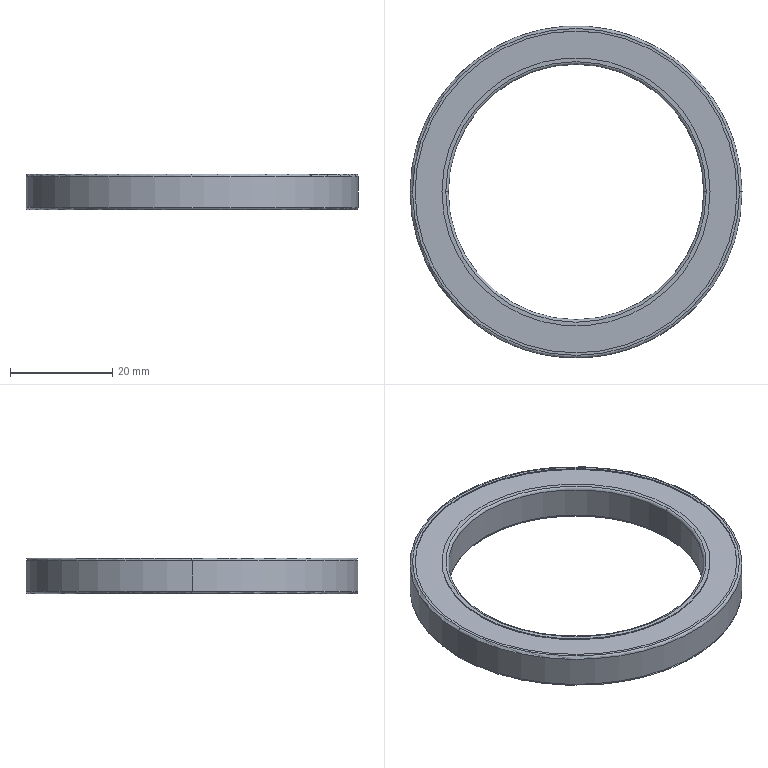Part | SolidWorks | features Extrusion 1, Fillet 1, ICE 1, MirrorPattern 1 | 1 solid | 26 faces | box 65 x 65 x 7 mm | volume 9064 mm3 | cylinder 12 | torus 8 | plane 6 | commonest cylinder face diameters 52.5 x4 63 x4 50 x2 65 x2
STEP:
#1=CARTESIAN_POINT('',(-25.5,0.,3.5));
#2=VERTEX_POINT('',#1);
#3=CARTESIAN_POINT('',(25.5,0.,3.5));
#4=VERTEX_POINT('',#3);
#5=CARTESIAN_POINT('',(0.,0.,3.5));
#6=DIRECTION('',(0.,0.,-1.));
#7=DIRECTION('',(1.,0.,0.));
#8=AXIS2_PLACEMENT_3D('',#5,#6,#7);
#9=CIRCLE('',#8,25.5);
#10=EDGE_CURVE('',#2,#4,#9,.T.);
#11=ORIENTED_EDGE('',*,*,#10,.F.);
#12=CARTESIAN_POINT('',(-25.,0.,3.));
#13=VERTEX_POINT('',#12);
#14=CARTESIAN_POINT('',(-25.5,0.,3.));
#15=DIRECTION('',(0.,1.,0.));
#16=DIRECTION('',(-1.,0.,0.));
#17=AXIS2_PLACEMENT_3D('',#14,#15,#16);
#18=CIRCLE('',#17,0.5);
#19=EDGE_CURVE('',#2,#13,#18,.T.);
#20=ORIENTED_EDGE('',*,*,#19,.T.);
#21=CARTESIAN_POINT('',(25.,0.,3.));
#22=VERTEX_POINT('',#21);
#23=CARTESIAN_POINT('',(0.,0.,3.));
#24=DIRECTION('',(0.,0.,1.));
#25=DIRECTION('',(1.,0.,0.));
#26=AXIS2_PLACEMENT_3D('',#23,#24,#25);
#27=CIRCLE('',#26,25.);
#28=EDGE_CURVE('',#22,#13,#27,.T.);
#29=ORIENTED_EDGE('',*,*,#28,.F.);
#30=CARTESIAN_POINT('',(25.5,0.,3.));
#31=DIRECTION('',(0.,-1.,0.));
#32=DIRECTION('',(0.,0.,-1.));
#33=AXIS2_PLACEMENT_3D('',#30,#31,#32);
#34=CIRCLE('',#33,0.5);
#35=EDGE_CURVE('',#4,#22,#34,.T.);
#36=ORIENTED_EDGE('',*,*,#35,.F.);
#37=EDGE_LOOP('',(#11,#20,#29,#36));
#38=FACE_OUTER_BOUND('',#37,.T.);
#39=CARTESIAN_POINT('',(0.,0.,3.));
#40=DIRECTION('',(0.,0.,1.));
#41=DIRECTION('',(1.,0.,0.));
#42=AXIS2_PLACEMENT_3D('',#39,#40,#41);
#43=TOROIDAL_SURFACE('',#42,25.5,0.5);
#44=ADVANCED_FACE('',(#38),#43,.T.);
#45=CARTESIAN_POINT('',(-25.,0.,-3.));
#46=VERTEX_POINT('',#45);
#47=CARTESIAN_POINT('',(25.,0.,-3.));
#48=VERTEX_POINT('',#47);
#49=CARTESIAN_POINT('',(0.,0.,-3.));
#50=DIRECTION('',(0.,0.,-1.));
#51=DIRECTION('',(1.,0.,0.));
#52=AXIS2_PLACEMENT_3D('',#49,#50,#51);
#53=CIRCLE('',#52,25.);
#54=EDGE_CURVE('',#46,#48,#53,.T.);
#55=ORIENTED_EDGE('',*,*,#54,.F.);
#56=CARTESIAN_POINT('',(-25.5,0.,-3.5));
#57=VERTEX_POINT('',#56);
#58=CARTESIAN_POINT('',(-25.5,0.,-3.));
#59=DIRECTION('',(0.,1.,0.));
#60=DIRECTION('',(-1.,0.,0.));
#61=AXIS2_PLACEMENT_3D('',#58,#59,#60);
#62=CIRCLE('',#61,0.5);
#63=EDGE_CURVE('',#46,#57,#62,.T.);
#64=ORIENTED_EDGE('',*,*,#63,.T.);
#65=CARTESIAN_POINT('',(25.5,0.,-3.5));
#66=VERTEX_POINT('',#65);
#67=CARTESIAN_POINT('',(0.,0.,-3.5));
#68=DIRECTION('',(0.,0.,1.));
#69=DIRECTION('',(1.,0.,0.));
#70=AXIS2_PLACEMENT_3D('',#67,#68,#69);
#71=CIRCLE('',#70,25.5);
#72=EDGE_CURVE('',#66,#57,#71,.T.);
#73=ORIENTED_EDGE('',*,*,#72,.F.);
#74=CARTESIAN_POINT('',(25.5,0.,-3.));
#75=DIRECTION('',(0.,-1.,0.));
#76=DIRECTION('',(0.,0.,-1.));
#77=AXIS2_PLACEMENT_3D('',#74,#75,#76);
#78=CIRCLE('',#77,0.5);
#79=EDGE_CURVE('',#48,#66,#78,.T.);
#80=ORIENTED_EDGE('',*,*,#79,.F.);
#81=EDGE_LOOP('',(#55,#64,#73,#80));
#82=FACE_OUTER_BOUND('',#81,.T.);
#83=CARTESIAN_POINT('',(0.,0.,-3.));
#84=DIRECTION('',(0.,0.,1.));
#85=DIRECTION('',(1.,0.,0.));
#86=AXIS2_PLACEMENT_3D('',#83,#84,#85);
#87=TOROIDAL_SURFACE('',#86,25.5,0.5);
#88=ADVANCED_FACE('',(#82),#87,.T.);
#89=CARTESIAN_POINT('',(-32.5,0.,3.));
#90=VERTEX_POINT('',#89);
#91=CARTESIAN_POINT('',(32.5,0.,3.));
#92=VERTEX_POINT('',#91);
#93=CARTESIAN_POINT('',(0.,0.,3.));
#94=DIRECTION('',(0.,0.,-1.));
#95=DIRECTION('',(1.,0.,0.));
#96=AXIS2_PLACEMENT_3D('',#93,#94,#95);
#97=CIRCLE('',#96,32.5);
#98=EDGE_CURVE('',#90,#92,#97,.T.);
#99=ORIENTED_EDGE('',*,*,#98,.F.);
#100=CARTESIAN_POINT('',(-32.,0.,3.5));
#101=VERTEX_POINT('',#100);
#102=CARTESIAN_POINT('',(-32.,0.,3.));
#103=DIRECTION('',(0.,1.,0.));
#104=DIRECTION('',(-1.,0.,0.));
#105=AXIS2_PLACEMENT_3D('',#102,#103,#104);
#106=CIRCLE('',#105,0.5);
#107=EDGE_CURVE('',#90,#101,#106,.T.);
#108=ORIENTED_EDGE('',*,*,#107,.T.);
#109=CARTESIAN_POINT('',(32.,0.,3.5));
#110=VERTEX_POINT('',#109);
#111=CARTESIAN_POINT('',(0.,0.,3.5));
#112=DIRECTION('',(0.,0.,1.));
#113=DIRECTION('',(1.,0.,0.));
#114=AXIS2_PLACEMENT_3D('',#111,#112,#113);
#115=CIRCLE('',#114,32.);
#116=EDGE_CURVE('',#110,#101,#115,.T.);
#117=ORIENTED_EDGE('',*,*,#116,.F.);
#118=CARTESIAN_POINT('',(32.,0.,3.));
#119=DIRECTION('',(0.,-1.,0.));
#120=DIRECTION('',(0.,0.,-1.));
#121=AXIS2_PLACEMENT_3D('',#118,#119,#120);
#122=CIRCLE('',#121,0.5);
#123=EDGE_CURVE('',#92,#110,#122,.T.);
#124=ORIENTED_EDGE('',*,*,#123,.F.);
#125=EDGE_LOOP('',(#99,#108,#117,#124));
#126=FACE_OUTER_BOUND('',#125,.T.);
#127=CARTESIAN_POINT('',(0.,0.,3.));
#128=DIRECTION('',(0.,0.,1.));
#129=DIRECTION('',(1.,0.,0.));
#130=AXIS2_PLACEMENT_3D('',#127,#128,#129);
#131=TOROIDAL_SURFACE('',#130,32.,0.5);
#132=ADVANCED_FACE('',(#126),#131,.T.);
#133=CARTESIAN_POINT('',(-32.,0.,-3.5));
#134=VERTEX_POINT('',#133);
#135=CARTESIAN_POINT('',(32.,0.,-3.5));
#136=VERTEX_POINT('',#135);
#137=CARTESIAN_POINT('',(0.,0.,-3.5));
#138=DIRECTION('',(0.,0.,-1.));
#139=DIRECTION('',(1.,0.,0.));
#140=AXIS2_PLACEMENT_3D('',#137,#138,#139);
#141=CIRCLE('',#140,32.);
#142=EDGE_CURVE('',#134,#136,#141,.T.);
#143=ORIENTED_EDGE('',*,*,#142,.F.);
#144=CARTESIAN_POINT('',(-32.5,0.,-3.));
#145=VERTEX_POINT('',#144);
#146=CARTESIAN_POINT('',(-32.,0.,-3.));
#147=DIRECTION('',(0.,1.,0.));
#148=DIRECTION('',(-1.,0.,0.));
#149=AXIS2_PLACEMENT_3D('',#146,#147,#148);
#150=CIRCLE('',#149,0.5);
#151=EDGE_CURVE('',#134,#145,#150,.T.);
#152=ORIENTED_EDGE('',*,*,#151,.T.);
#153=CARTESIAN_POINT('',(32.5,0.,-3.));
#154=VERTEX_POINT('',#153);
#155=CARTESIAN_POINT('',(0.,0.,-3.));
#156=DIRECTION('',(0.,0.,1.));
#157=DIRECTION('',(1.,0.,0.));
#158=AXIS2_PLACEMENT_3D('',#155,#156,#157);
#159=CIRCLE('',#158,32.5);
#160=EDGE_CURVE('',#154,#145,#159,.T.);
#161=ORIENTED_EDGE('',*,*,#160,.F.);
#162=CARTESIAN_POINT('',(32.,0.,-3.));
#163=DIRECTION('',(0.,-1.,0.));
#164=DIRECTION('',(0.,0.,-1.));
#165=AXIS2_PLACEMENT_3D('',#162,#163,#164);
#166=CIRCLE('',#165,0.5);
#167=EDGE_CURVE('',#136,#154,#166,.T.);
#168=ORIENTED_EDGE('',*,*,#167,.F.);
#169=EDGE_LOOP('',(#143,#152,#161,#168));
#170=FACE_OUTER_BOUND('',#169,.T.);
#171=CARTESIAN_POINT('',(0.,0.,-3.));
#172=DIRECTION('',(0.,0.,1.));
#173=DIRECTION('',(1.,0.,0.));
#174=AXIS2_PLACEMENT_3D('',#171,#172,#173);
#175=TOROIDAL_SURFACE('',#174,32.,0.5);
#176=ADVANCED_FACE('',(#170),#175,.T.);
#177=CARTESIAN_POINT('',(26.25,0.,-3.3));
#178=VERTEX_POINT('',#177);
#179=CARTESIAN_POINT('',(-26.25,0.,-3.3));
#180=VERTEX_POINT('',#179);
#181=CARTESIAN_POINT('',(0.,0.,-3.3));
#182=DIRECTION('',(0.,0.,1.));
#183=DIRECTION('',(1.,0.,0.));
#184=AXIS2_PLACEMENT_3D('',#181,#182,#183);
#185=CIRCLE('',#184,26.25);
#186=EDGE_CURVE('',#178,#180,#185,.T.);
#187=ORIENTED_EDGE('',*,*,#186,.F.);
#188=CARTESIAN_POINT('',(26.25,0.,-3.5));
#189=VERTEX_POINT('',#188);
#190=CARTESIAN_POINT('',(26.25,0.,-3.3));
#191=DIRECTION('',(0.,0.,-1.));
#192=VECTOR('',#191,1000.);
#193=LINE('',#190,#192);
#194=EDGE_CURVE('',#178,#189,#193,.T.);
#195=ORIENTED_EDGE('',*,*,#194,.T.);
#196=CARTESIAN_POINT('',(-26.25,0.,-3.5));
#197=VERTEX_POINT('',#196);
#198=CARTESIAN_POINT('',(0.,0.,-3.5));
#199=DIRECTION('',(0.,0.,1.));
#200=DIRECTION('',(1.,0.,0.));
#201=AXIS2_PLACEMENT_3D('',#198,#199,#200);
#202=CIRCLE('',#201,26.25);
#203=EDGE_CURVE('',#189,#197,#202,.T.);
#204=ORIENTED_EDGE('',*,*,#203,.T.);
#205=CARTESIAN_POINT('',(-26.25,0.,-3.3));
#206=DIRECTION('',(0.,0.,-1.));
#207=VECTOR('',#206,1000.);
#208=LINE('',#205,#207);
#209=EDGE_CURVE('',#180,#197,#208,.T.);
#210=ORIENTED_EDGE('',*,*,#209,.F.);
#211=EDGE_LOOP('',(#187,#195,#204,#210));
#212=FACE_OUTER_BOUND('',#211,.T.);
#213=CARTESIAN_POINT('',(0.,0.,-3.3));
#214=DIRECTION('',(0.,0.,-1.));
#215=DIRECTION('',(-1.,0.,0.));
#216=AXIS2_PLACEMENT_3D('',#213,#214,#215);
#217=CYLINDRICAL_SURFACE('',#216,26.25);
#218=ADVANCED_FACE('',(#212),#217,.T.);
#219=CARTESIAN_POINT('',(-31.5,0.,-3.3));
#220=VERTEX_POINT('',#219);
#221=CARTESIAN_POINT('',(31.5,0.,-3.3));
#222=VERTEX_POINT('',#221);
#223=CARTESIAN_POINT('',(0.,0.,-3.3));
#224=DIRECTION('',(0.,0.,1.));
#225=DIRECTION('',(1.,0.,0.));
#226=AXIS2_PLACEMENT_3D('',#223,#224,#225);
#227=CIRCLE('',#226,31.5);
#228=EDGE_CURVE('',#220,#222,#227,.T.);
#229=ORIENTED_EDGE('',*,*,#228,.T.);
#230=CARTESIAN_POINT('',(31.5,0.,-3.5));
#231=VERTEX_POINT('',#230);
#232=CARTESIAN_POINT('',(31.5,0.,-3.3));
#233=DIRECTION('',(0.,0.,-1.));
#234=VECTOR('',#233,1000.);
#235=LINE('',#232,#234);
#236=EDGE_CURVE('',#222,#231,#235,.T.);
#237=ORIENTED_EDGE('',*,*,#236,.T.);
#238=CARTESIAN_POINT('',(-31.5,0.,-3.5));
#239=VERTEX_POINT('',#238);
#240=CARTESIAN_POINT('',(0.,0.,-3.5));
#241=DIRECTION('',(0.,0.,1.));
#242=DIRECTION('',(1.,0.,0.));
#243=AXIS2_PLACEMENT_3D('',#240,#241,#242);
#244=CIRCLE('',#243,31.5);
#245=EDGE_CURVE('',#239,#231,#244,.T.);
#246=ORIENTED_EDGE('',*,*,#245,.F.);
#247=CARTESIAN_POINT('',(-31.5,0.,-3.3));
#248=DIRECTION('',(0.,0.,-1.));
#249=VECTOR('',#248,1000.);
#250=LINE('',#247,#249);
#251=EDGE_CURVE('',#220,#239,#250,.T.);
#252=ORIENTED_EDGE('',*,*,#251,.F.);
#253=EDGE_LOOP('',(#229,#237,#246,#252));
#254=FACE_OUTER_BOUND('',#253,.T.);
#255=CARTESIAN_POINT('',(0.,0.,-3.3));
#256=DIRECTION('',(0.,0.,-1.));
#257=DIRECTION('',(-1.,0.,0.));
#258=AXIS2_PLACEMENT_3D('',#255,#256,#257);
#259=CYLINDRICAL_SURFACE('',#258,31.5);
#260=ADVANCED_FACE('',(#254),#259,.F.);
#261=CARTESIAN_POINT('',(26.25,0.,3.3));
#262=VERTEX_POINT('',#261);
#263=CARTESIAN_POINT('',(-26.25,0.,3.3));
#264=VERTEX_POINT('',#263);
#265=CARTESIAN_POINT('',(0.,0.,3.3));
#266=DIRECTION('',(0.,0.,1.));
#267=DIRECTION('',(1.,0.,0.));
#268=AXIS2_PLACEMENT_3D('',#265,#266,#267);
#269=CIRCLE('',#268,26.25);
#270=EDGE_CURVE('',#262,#264,#269,.T.);
#271=ORIENTED_EDGE('',*,*,#270,.T.);
#272=CARTESIAN_POINT('',(-26.25,0.,3.5));
#273=VERTEX_POINT('',#272);
#274=CARTESIAN_POINT('',(-26.25,0.,3.3));
#275=DIRECTION('',(0.,0.,1.));
#276=VECTOR('',#275,1000.);
#277=LINE('',#274,#276);
#278=EDGE_CURVE('',#264,#273,#277,.T.);
#279=ORIENTED_EDGE('',*,*,#278,.T.);
#280=CARTESIAN_POINT('',(26.25,0.,3.5));
#281=VERTEX_POINT('',#280);
#282=CARTESIAN_POINT('',(0.,0.,3.5));
#283=DIRECTION('',(0.,0.,1.));
#284=DIRECTION('',(1.,0.,0.));
#285=AXIS2_PLACEMENT_3D('',#282,#283,#284);
#286=CIRCLE('',#285,26.25);
#287=EDGE_CURVE('',#281,#273,#286,.T.);
#288=ORIENTED_EDGE('',*,*,#287,.F.);
#289=CARTESIAN_POINT('',(26.25,0.,3.3));
#290=DIRECTION('',(0.,0.,1.));
#291=VECTOR('',#290,1000.);
#292=LINE('',#289,#291);
#293=EDGE_CURVE('',#262,#281,#292,.T.);
#294=ORIENTED_EDGE('',*,*,#293,.F.);
#295=EDGE_LOOP('',(#271,#279,#288,#294));
#296=FACE_OUTER_BOUND('',#295,.T.);
#297=CARTESIAN_POINT('',(0.,0.,3.3));
#298=DIRECTION('',(0.,0.,1.));
#299=DIRECTION('',(1.,0.,0.));
#300=AXIS2_PLACEMENT_3D('',#297,#298,#299);
#301=CYLINDRICAL_SURFACE('',#300,26.25);
#302=ADVANCED_FACE('',(#296),#301,.T.);
#303=CARTESIAN_POINT('',(-31.5,0.,3.3));
#304=VERTEX_POINT('',#303);
#305=CARTESIAN_POINT('',(31.5,0.,3.3));
#306=VERTEX_POINT('',#305);
#307=CARTESIAN_POINT('',(0.,0.,3.3));
#308=DIRECTION('',(0.,0.,1.));
#309=DIRECTION('',(1.,0.,0.));
#310=AXIS2_PLACEMENT_3D('',#307,#308,#309);
#311=CIRCLE('',#310,31.5);
#312=EDGE_CURVE('',#304,#306,#311,.T.);
#313=ORIENTED_EDGE('',*,*,#312,.F.);
#314=CARTESIAN_POINT('',(-31.5,0.,3.5));
#315=VERTEX_POINT('',#314);
#316=CARTESIAN_POINT('',(-31.5,0.,3.3));
#317=DIRECTION('',(0.,0.,1.));
#318=VECTOR('',#317,1000.);
#319=LINE('',#316,#318);
#320=EDGE_CURVE('',#304,#315,#319,.T.);
#321=ORIENTED_EDGE('',*,*,#320,.T.);
#322=CARTESIAN_POINT('',(31.5,0.,3.5));
#323=VERTEX_POINT('',#322);
#324=CARTESIAN_POINT('',(0.,0.,3.5));
#325=DIRECTION('',(0.,0.,1.));
#326=DIRECTION('',(1.,0.,0.));
#327=AXIS2_PLACEMENT_3D('',#324,#325,#326);
#328=CIRCLE('',#327,31.5);
#329=EDGE_CURVE('',#315,#323,#328,.T.);
#330=ORIENTED_EDGE('',*,*,#329,.T.);
#331=CARTESIAN_POINT('',(31.5,0.,3.3));
#332=DIRECTION('',(0.,0.,1.));
#333=VECTOR('',#332,1000.);
#334=LINE('',#331,#333);
#335=EDGE_CURVE('',#306,#323,#334,.T.);
#336=ORIENTED_EDGE('',*,*,#335,.F.);
#337=EDGE_LOOP('',(#313,#321,#330,#336));
#338=FACE_OUTER_BOUND('',#337,.T.);
#339=CARTESIAN_POINT('',(0.,0.,3.3));
#340=DIRECTION('',(0.,0.,1.));
#341=DIRECTION('',(1.,0.,0.));
#342=AXIS2_PLACEMENT_3D('',#339,#340,#341);
#343=CYLINDRICAL_SURFACE('',#342,31.5);
#344=ADVANCED_FACE('',(#338),#343,.F.);
#345=CARTESIAN_POINT('',(0.,0.,3.));
#346=DIRECTION('',(0.,0.,1.));
#347=DIRECTION('',(1.,0.,0.));
#348=AXIS2_PLACEMENT_3D('',#345,#346,#347);
#349=CIRCLE('',#348,25.);
#350=EDGE_CURVE('',#13,#22,#349,.T.);
#351=ORIENTED_EDGE('',*,*,#350,.T.);
#352=CARTESIAN_POINT('',(25.,0.,3.5));
#353=DIRECTION('',(0.,0.,-1.));
#354=VECTOR('',#353,1000.);
#355=LINE('',#352,#354);
#356=EDGE_CURVE('',#22,#48,#355,.T.);
#357=ORIENTED_EDGE('',*,*,#356,.T.);
#358=CARTESIAN_POINT('',(0.,0.,-3.));
#359=DIRECTION('',(0.,0.,-1.));
#360=DIRECTION('',(1.,0.,0.));
#361=AXIS2_PLACEMENT_3D('',#358,#359,#360);
#362=CIRCLE('',#361,25.);
#363=EDGE_CURVE('',#48,#46,#362,.T.);
#364=ORIENTED_EDGE('',*,*,#363,.T.);
#365=CARTESIAN_POINT('',(-25.,0.,3.5));
#366=DIRECTION('',(0.,0.,-1.));
#367=VECTOR('',#366,1000.);
#368=LINE('',#365,#367);
#369=EDGE_CURVE('',#13,#46,#368,.T.);
#370=ORIENTED_EDGE('',*,*,#369,.F.);
#371=EDGE_LOOP('',(#351,#357,#364,#370));
#372=FACE_OUTER_BOUND('',#371,.T.);
#373=CARTESIAN_POINT('',(0.,0.,3.5));
#374=DIRECTION('',(0.,0.,-1.));
#375=DIRECTION('',(-1.,0.,0.));
#376=AXIS2_PLACEMENT_3D('',#373,#374,#375);
#377=CYLINDRICAL_SURFACE('',#376,25.);
#378=ADVANCED_FACE('',(#372),#377,.F.);
#379=ORIENTED_EDGE('',*,*,#98,.T.);
#380=CARTESIAN_POINT('',(32.5,0.,3.5));
#381=DIRECTION('',(0.,0.,-1.));
#382=VECTOR('',#381,1000.);
#383=LINE('',#380,#382);
#384=EDGE_CURVE('',#92,#154,#383,.T.);
#385=ORIENTED_EDGE('',*,*,#384,.T.);
#386=ORIENTED_EDGE('',*,*,#160,.T.);
#387=CARTESIAN_POINT('',(-32.5,0.,3.5));
#388=DIRECTION('',(0.,0.,-1.));
#389=VECTOR('',#388,1000.);
#390=LINE('',#387,#389);
#391=EDGE_CURVE('',#90,#145,#390,.T.);
#392=ORIENTED_EDGE('',*,*,#391,.F.);
#393=EDGE_LOOP('',(#379,#385,#386,#392));
#394=FACE_OUTER_BOUND('',#393,.T.);
#395=CARTESIAN_POINT('',(0.,0.,3.5));
#396=DIRECTION('',(0.,0.,-1.));
#397=DIRECTION('',(-1.,0.,0.));
#398=AXIS2_PLACEMENT_3D('',#395,#396,#397);
#399=CYLINDRICAL_SURFACE('',#398,32.5);
#400=ADVANCED_FACE('',(#394),#399,.T.);
#401=CARTESIAN_POINT('',(0.,0.,-3.5));
#402=DIRECTION('',(0.,0.,-1.));
#403=DIRECTION('',(1.,0.,0.));
#404=AXIS2_PLACEMENT_3D('',#401,#402,#403);
#405=CIRCLE('',#404,32.);
#406=EDGE_CURVE('',#136,#134,#405,.T.);
#407=ORIENTED_EDGE('',*,*,#406,.T.);
#408=ORIENTED_EDGE('',*,*,#142,.T.);
#409=EDGE_LOOP('',(#407,#408));
#410=FACE_OUTER_BOUND('',#409,.T.);
#411=ORIENTED_EDGE('',*,*,#245,.T.);
#412=CARTESIAN_POINT('',(0.,0.,-3.5));
#413=DIRECTION('',(0.,0.,1.));
#414=DIRECTION('',(1.,0.,0.));
#415=AXIS2_PLACEMENT_3D('',#412,#413,#414);
#416=CIRCLE('',#415,31.5);
#417=EDGE_CURVE('',#231,#239,#416,.T.);
#418=ORIENTED_EDGE('',*,*,#417,.T.);
#419=EDGE_LOOP('',(#411,#418));
#420=FACE_BOUND('',#419,.T.);
#421=CARTESIAN_POINT('',(0.,0.,-3.5));
#422=DIRECTION('',(0.,0.,1.));
#423=DIRECTION('',(1.,0.,0.));
#424=AXIS2_PLACEMENT_3D('',#421,#422,#423);
#425=PLANE('',#424);
#426=ADVANCED_FACE('',(#410,#420),#425,.F.);
#427=CARTESIAN_POINT('',(0.,0.,3.5));
#428=DIRECTION('',(0.,0.,-1.));
#429=DIRECTION('',(1.,0.,0.));
#430=AXIS2_PLACEMENT_3D('',#427,#428,#429);
#431=CIRCLE('',#430,25.5);
#432=EDGE_CURVE('',#4,#2,#431,.T.);
#433=ORIENTED_EDGE('',*,*,#432,.T.);
#434=ORIENTED_EDGE('',*,*,#10,.T.);
#435=EDGE_LOOP('',(#433,#434));
#436=FACE_BOUND('',#435,.T.);
#437=ORIENTED_EDGE('',*,*,#287,.T.);
#438=CARTESIAN_POINT('',(0.,0.,3.5));
#439=DIRECTION('',(0.,0.,1.));
#440=DIRECTION('',(1.,0.,0.));
#441=AXIS2_PLACEMENT_3D('',#438,#439,#440);
#442=CIRCLE('',#441,26.25);
#443=EDGE_CURVE('',#273,#281,#442,.T.);
#444=ORIENTED_EDGE('',*,*,#443,.T.);
#445=EDGE_LOOP('',(#437,#444));
#446=FACE_OUTER_BOUND('',#445,.T.);
#447=CARTESIAN_POINT('',(0.,0.,3.5));
#448=DIRECTION('',(0.,0.,1.));
#449=DIRECTION('',(1.,0.,0.));
#450=AXIS2_PLACEMENT_3D('',#447,#448,#449);
#451=PLANE('',#450);
#452=ADVANCED_FACE('',(#436,#446),#451,.T.);
#453=ORIENTED_EDGE('',*,*,#116,.T.);
#454=CARTESIAN_POINT('',(0.,0.,3.5));
#455=DIRECTION('',(0.,0.,1.));
#456=DIRECTION('',(1.,0.,0.));
#457=AXIS2_PLACEMENT_3D('',#454,#455,#456);
#458=CIRCLE('',#457,32.);
#459=EDGE_CURVE('',#101,#110,#458,.T.);
#460=ORIENTED_EDGE('',*,*,#459,.T.);
#461=EDGE_LOOP('',(#453,#460));
#462=FACE_OUTER_BOUND('',#461,.T.);
#463=CARTESIAN_POINT('',(0.,0.,3.5));
#464=DIRECTION('',(0.,0.,1.));
#465=DIRECTION('',(1.,0.,0.));
#466=AXIS2_PLACEMENT_3D('',#463,#464,#465);
#467=CIRCLE('',#466,31.5);
#468=EDGE_CURVE('',#323,#315,#467,.T.);
#469=ORIENTED_EDGE('',*,*,#468,.F.);
#470=ORIENTED_EDGE('',*,*,#329,.F.);
#471=EDGE_LOOP('',(#469,#470));
#472=FACE_BOUND('',#471,.T.);
#473=CARTESIAN_POINT('',(0.,0.,3.5));
#474=DIRECTION('',(0.,0.,1.));
#475=DIRECTION('',(1.,0.,0.));
#476=AXIS2_PLACEMENT_3D('',#473,#474,#475);
#477=PLANE('',#476);
#478=ADVANCED_FACE('',(#462,#472),#477,.T.);
#479=ORIENTED_EDGE('',*,*,#72,.T.);
#480=CARTESIAN_POINT('',(0.,0.,-3.5));
#481=DIRECTION('',(0.,0.,1.));
#482=DIRECTION('',(1.,0.,0.));
#483=AXIS2_PLACEMENT_3D('',#480,#481,#482);
#484=CIRCLE('',#483,25.5);
#485=EDGE_CURVE('',#57,#66,#484,.T.);
#486=ORIENTED_EDGE('',*,*,#485,.T.);
#487=EDGE_LOOP('',(#479,#486));
#488=FACE_BOUND('',#487,.T.);
#489=CARTESIAN_POINT('',(0.,0.,-3.5));
#490=DIRECTION('',(0.,0.,1.));
#491=DIRECTION('',(1.,0.,0.));
#492=AXIS2_PLACEMENT_3D('',#489,#490,#491);
#493=CIRCLE('',#492,26.25);
#494=EDGE_CURVE('',#197,#189,#493,.T.);
#495=ORIENTED_EDGE('',*,*,#494,.F.);
#496=ORIENTED_EDGE('',*,*,#203,.F.);
#497=EDGE_LOOP('',(#495,#496));
#498=FACE_OUTER_BOUND('',#497,.T.);
#499=CARTESIAN_POINT('',(0.,0.,-3.5));
#500=DIRECTION('',(0.,0.,1.));
#501=DIRECTION('',(1.,0.,0.));
#502=AXIS2_PLACEMENT_3D('',#499,#500,#501);
#503=PLANE('',#502);
#504=ADVANCED_FACE('',(#488,#498),#503,.F.);
#505=ORIENTED_EDGE('',*,*,#384,.F.);
#506=CARTESIAN_POINT('',(0.,0.,3.));
#507=DIRECTION('',(0.,0.,-1.));
#508=DIRECTION('',(1.,0.,0.));
#509=AXIS2_PLACEMENT_3D('',#506,#507,#508);
#510=CIRCLE('',#509,32.5);
#511=EDGE_CURVE('',#92,#90,#510,.T.);
#512=ORIENTED_EDGE('',*,*,#511,.T.);
#513=ORIENTED_EDGE('',*,*,#391,.T.);
#514=CARTESIAN_POINT('',(0.,0.,-3.));
#515=DIRECTION('',(0.,0.,1.));
#516=DIRECTION('',(1.,0.,0.));
#517=AXIS2_PLACEMENT_3D('',#514,#515,#516);
#518=CIRCLE('',#517,32.5);
#519=EDGE_CURVE('',#145,#154,#518,.T.);
#520=ORIENTED_EDGE('',*,*,#519,.T.);
#521=EDGE_LOOP('',(#505,#512,#513,#520));
#522=FACE_OUTER_BOUND('',#521,.T.);
#523=CARTESIAN_POINT('',(0.,0.,3.5));
#524=DIRECTION('',(0.,0.,-1.));
#525=DIRECTION('',(-1.,0.,0.));
#526=AXIS2_PLACEMENT_3D('',#523,#524,#525);
#527=CYLINDRICAL_SURFACE('',#526,32.5);
#528=ADVANCED_FACE('',(#522),#527,.T.);
#529=ORIENTED_EDGE('',*,*,#356,.F.);
#530=ORIENTED_EDGE('',*,*,#28,.T.);
#531=ORIENTED_EDGE('',*,*,#369,.T.);
#532=ORIENTED_EDGE('',*,*,#54,.T.);
#533=EDGE_LOOP('',(#529,#530,#531,#532));
#534=FACE_OUTER_BOUND('',#533,.T.);
#535=CARTESIAN_POINT('',(0.,0.,3.5));
#536=DIRECTION('',(0.,0.,-1.));
#537=DIRECTION('',(-1.,0.,0.));
#538=AXIS2_PLACEMENT_3D('',#535,#536,#537);
#539=CYLINDRICAL_SURFACE('',#538,25.);
#540=ADVANCED_FACE('',(#534),#539,.F.);
#541=ORIENTED_EDGE('',*,*,#320,.F.);
#542=CARTESIAN_POINT('',(0.,0.,3.3));
#543=DIRECTION('',(0.,0.,1.));
#544=DIRECTION('',(1.,0.,0.));
#545=AXIS2_PLACEMENT_3D('',#542,#543,#544);
#546=CIRCLE('',#545,31.5);
#547=EDGE_CURVE('',#306,#304,#546,.T.);
#548=ORIENTED_EDGE('',*,*,#547,.F.);
#549=ORIENTED_EDGE('',*,*,#335,.T.);
#550=ORIENTED_EDGE('',*,*,#468,.T.);
#551=EDGE_LOOP('',(#541,#548,#549,#550));
#552=FACE_OUTER_BOUND('',#551,.T.);
#553=CARTESIAN_POINT('',(0.,0.,3.3));
#554=DIRECTION('',(0.,0.,1.));
#555=DIRECTION('',(1.,0.,0.));
#556=AXIS2_PLACEMENT_3D('',#553,#554,#555);
#557=CYLINDRICAL_SURFACE('',#556,31.5);
#558=ADVANCED_FACE('',(#552),#557,.F.);
#559=ORIENTED_EDGE('',*,*,#270,.F.);
#560=CARTESIAN_POINT('',(0.,0.,3.3));
#561=DIRECTION('',(0.,0.,1.));
#562=DIRECTION('',(1.,0.,0.));
#563=AXIS2_PLACEMENT_3D('',#560,#561,#562);
#564=CIRCLE('',#563,26.25);
#565=EDGE_CURVE('',#264,#262,#564,.T.);
#566=ORIENTED_EDGE('',*,*,#565,.F.);
#567=EDGE_LOOP('',(#559,#566));
#568=FACE_BOUND('',#567,.T.);
#569=ORIENTED_EDGE('',*,*,#547,.T.);
#570=ORIENTED_EDGE('',*,*,#312,.T.);
#571=EDGE_LOOP('',(#569,#570));
#572=FACE_OUTER_BOUND('',#571,.T.);
#573=CARTESIAN_POINT('',(0.,0.,3.3));
#574=DIRECTION('',(0.,0.,1.));
#575=DIRECTION('',(1.,0.,0.));
#576=AXIS2_PLACEMENT_3D('',#573,#574,#575);
#577=PLANE('',#576);
#578=ADVANCED_FACE('',(#568,#572),#577,.T.);
#579=ORIENTED_EDGE('',*,*,#278,.F.);
#580=ORIENTED_EDGE('',*,*,#565,.T.);
#581=ORIENTED_EDGE('',*,*,#293,.T.);
#582=ORIENTED_EDGE('',*,*,#443,.F.);
#583=EDGE_LOOP('',(#579,#580,#581,#582));
#584=FACE_OUTER_BOUND('',#583,.T.);
#585=CARTESIAN_POINT('',(0.,0.,3.3));
#586=DIRECTION('',(0.,0.,1.));
#587=DIRECTION('',(1.,0.,0.));
#588=AXIS2_PLACEMENT_3D('',#585,#586,#587);
#589=CYLINDRICAL_SURFACE('',#588,26.25);
#590=ADVANCED_FACE('',(#584),#589,.T.);
#591=ORIENTED_EDGE('',*,*,#228,.F.);
#592=CARTESIAN_POINT('',(0.,0.,-3.3));
#593=DIRECTION('',(0.,0.,1.));
#594=DIRECTION('',(1.,0.,0.));
#595=AXIS2_PLACEMENT_3D('',#592,#593,#594);
#596=CIRCLE('',#595,31.5);
#597=EDGE_CURVE('',#222,#220,#596,.T.);
#598=ORIENTED_EDGE('',*,*,#597,.F.);
#599=EDGE_LOOP('',(#591,#598));
#600=FACE_OUTER_BOUND('',#599,.T.);
#601=CARTESIAN_POINT('',(0.,0.,-3.3));
#602=DIRECTION('',(0.,0.,1.));
#603=DIRECTION('',(1.,0.,0.));
#604=AXIS2_PLACEMENT_3D('',#601,#602,#603);
#605=CIRCLE('',#604,26.25);
#606=EDGE_CURVE('',#180,#178,#605,.T.);
#607=ORIENTED_EDGE('',*,*,#606,.T.);
#608=ORIENTED_EDGE('',*,*,#186,.T.);
#609=EDGE_LOOP('',(#607,#608));
#610=FACE_BOUND('',#609,.T.);
#611=CARTESIAN_POINT('',(0.,0.,-3.3));
#612=DIRECTION('',(0.,0.,-1.));
#613=DIRECTION('',(1.,0.,0.));
#614=AXIS2_PLACEMENT_3D('',#611,#612,#613);
#615=PLANE('',#614);
#616=ADVANCED_FACE('',(#600,#610),#615,.T.);
#617=ORIENTED_EDGE('',*,*,#236,.F.);
#618=ORIENTED_EDGE('',*,*,#597,.T.);
#619=ORIENTED_EDGE('',*,*,#251,.T.);
#620=ORIENTED_EDGE('',*,*,#417,.F.);
#621=EDGE_LOOP('',(#617,#618,#619,#620));
#622=FACE_OUTER_BOUND('',#621,.T.);
#623=CARTESIAN_POINT('',(0.,0.,-3.3));
#624=DIRECTION('',(0.,0.,-1.));
#625=DIRECTION('',(-1.,0.,0.));
#626=AXIS2_PLACEMENT_3D('',#623,#624,#625);
#627=CYLINDRICAL_SURFACE('',#626,31.5);
#628=ADVANCED_FACE('',(#622),#627,.F.);
#629=ORIENTED_EDGE('',*,*,#194,.F.);
#630=ORIENTED_EDGE('',*,*,#606,.F.);
#631=ORIENTED_EDGE('',*,*,#209,.T.);
#632=ORIENTED_EDGE('',*,*,#494,.T.);
#633=EDGE_LOOP('',(#629,#630,#631,#632));
#634=FACE_OUTER_BOUND('',#633,.T.);
#635=CARTESIAN_POINT('',(0.,0.,-3.3));
#636=DIRECTION('',(0.,0.,-1.));
#637=DIRECTION('',(-1.,0.,0.));
#638=AXIS2_PLACEMENT_3D('',#635,#636,#637);
#639=CYLINDRICAL_SURFACE('',#638,26.25);
#640=ADVANCED_FACE('',(#634),#639,.T.);
#641=ORIENTED_EDGE('',*,*,#151,.F.);
#642=ORIENTED_EDGE('',*,*,#406,.F.);
#643=ORIENTED_EDGE('',*,*,#167,.T.);
#644=ORIENTED_EDGE('',*,*,#519,.F.);
#645=EDGE_LOOP('',(#641,#642,#643,#644));
#646=FACE_OUTER_BOUND('',#645,.T.);
#647=CARTESIAN_POINT('',(0.,0.,-3.));
#648=DIRECTION('',(0.,0.,1.));
#649=DIRECTION('',(1.,0.,0.));
#650=AXIS2_PLACEMENT_3D('',#647,#648,#649);
#651=TOROIDAL_SURFACE('',#650,32.,0.5);
#652=ADVANCED_FACE('',(#646),#651,.T.);
#653=ORIENTED_EDGE('',*,*,#107,.F.);
#654=ORIENTED_EDGE('',*,*,#511,.F.);
#655=ORIENTED_EDGE('',*,*,#123,.T.);
#656=ORIENTED_EDGE('',*,*,#459,.F.);
#657=EDGE_LOOP('',(#653,#654,#655,#656));
#658=FACE_OUTER_BOUND('',#657,.T.);
#659=CARTESIAN_POINT('',(0.,0.,3.));
#660=DIRECTION('',(0.,0.,1.));
#661=DIRECTION('',(1.,0.,0.));
#662=AXIS2_PLACEMENT_3D('',#659,#660,#661);
#663=TOROIDAL_SURFACE('',#662,32.,0.5);
#664=ADVANCED_FACE('',(#658),#663,.T.);
#665=ORIENTED_EDGE('',*,*,#63,.F.);
#666=ORIENTED_EDGE('',*,*,#363,.F.);
#667=ORIENTED_EDGE('',*,*,#79,.T.);
#668=ORIENTED_EDGE('',*,*,#485,.F.);
#669=EDGE_LOOP('',(#665,#666,#667,#668));
#670=FACE_OUTER_BOUND('',#669,.T.);
#671=CARTESIAN_POINT('',(0.,0.,-3.));
#672=DIRECTION('',(0.,0.,1.));
#673=DIRECTION('',(1.,0.,0.));
#674=AXIS2_PLACEMENT_3D('',#671,#672,#673);
#675=TOROIDAL_SURFACE('',#674,25.5,0.5);
#676=ADVANCED_FACE('',(#670),#675,.T.);
#677=ORIENTED_EDGE('',*,*,#19,.F.);
#678=ORIENTED_EDGE('',*,*,#432,.F.);
#679=ORIENTED_EDGE('',*,*,#35,.T.);
#680=ORIENTED_EDGE('',*,*,#350,.F.);
#681=EDGE_LOOP('',(#677,#678,#679,#680));
#682=FACE_OUTER_BOUND('',#681,.T.);
#683=CARTESIAN_POINT('',(0.,0.,3.));
#684=DIRECTION('',(0.,0.,1.));
#685=DIRECTION('',(1.,0.,0.));
#686=AXIS2_PLACEMENT_3D('',#683,#684,#685);
#687=TOROIDAL_SURFACE('',#686,25.5,0.5);
#688=ADVANCED_FACE('',(#682),#687,.T.);
#689=CLOSED_SHELL('',(#44,#88,#132,#176,#218,#260,#302,#344,#378,#400,#426,#452,#478,#504,#528,#540,#558,#578,#590,#616,#628,#640,#652,#664,#676,#688));
#690=MANIFOLD_SOLID_BREP('',#689);
#691=CARTESIAN_POINT('',(0.,0.,0.));
#692=DIRECTION('',(0.,0.,1.));
#693=DIRECTION('',(1.,0.,0.));
#694=AXIS2_PLACEMENT_3D('',#691,#692,#693);
#695=(LENGTH_UNIT()NAMED_UNIT(*)SI_UNIT(.MILLI.,.METRE.));
#696=UNCERTAINTY_MEASURE_WITH_UNIT(LENGTH_MEASURE(0.00001),#695,'','');
#697=(NAMED_UNIT(*)PLANE_ANGLE_UNIT()SI_UNIT($,.RADIAN.));
#698=(NAMED_UNIT(*)SI_UNIT($,.STERADIAN.)SOLID_ANGLE_UNIT());
#699=(GEOMETRIC_REPRESENTATION_CONTEXT(3)GLOBAL_UNCERTAINTY_ASSIGNED_CONTEXT((#696))GLOBAL_UNIT_ASSIGNED_CONTEXT((#695,#697,#698))REPRESENTATION_CONTEXT('',''));
#700=ADVANCED_BREP_SHAPE_REPRESENTATION('',(#690,#694),#699);